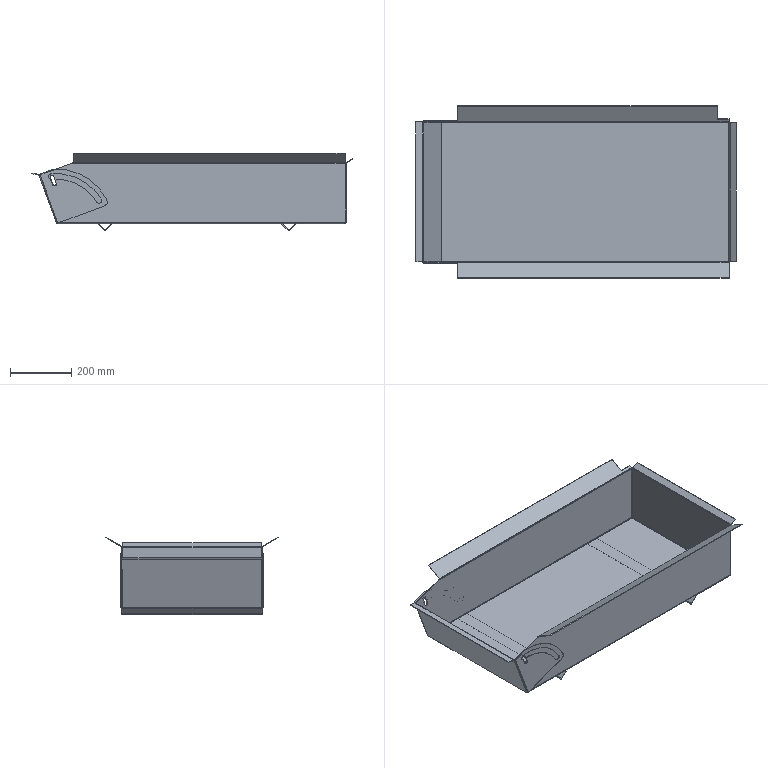Part | SolidWorks | features BaseBody 4 | 4 solids | 134 faces | box 1048 x 561.923 x 252.092 mm | volume 2371643 mm3 | plane 72 | cylinder 56 | spline 6 | commonest cylinder face diameters 8 x15 4 x9 11 x6 18 x6 10 x4 30 x4